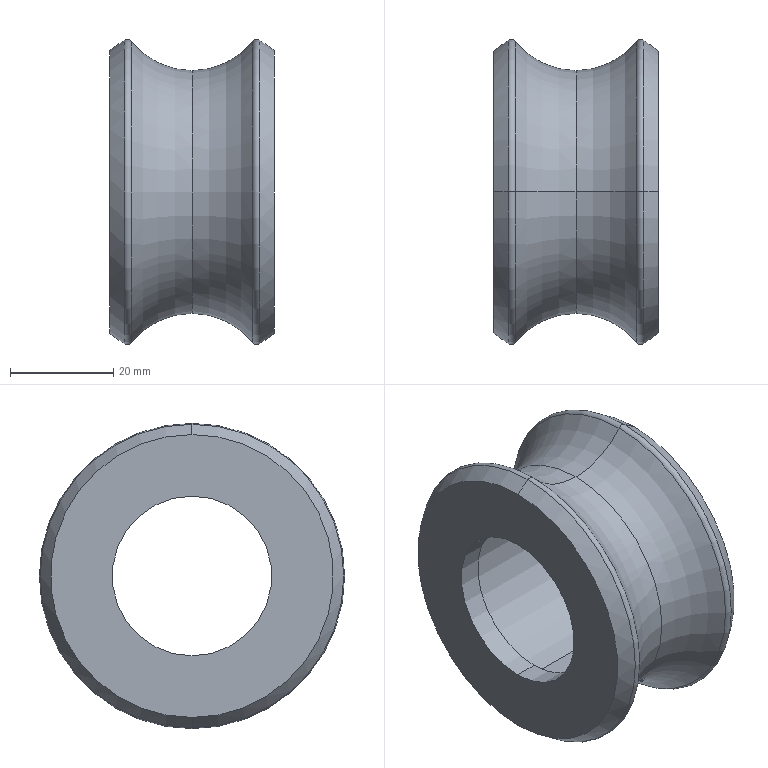Part | STEP file | RODAJA D29 | 1 solid | 29 faces | box 32 x 59.25 x 59.25 mm | volume 39424 mm3 | torus 10 | cylinder 8 | cone 6 | plane 5 | commonest cylinder face diameters 35 x4 31 x2 37.2 x2
STEP:
#1=CARTESIAN_POINT('',(-11.807,0.,-26.413));
#2=VERTEX_POINT('',#1);
#3=CARTESIAN_POINT('',(0.,0.,-32.1));
#4=VERTEX_POINT('',#3);
#5=CARTESIAN_POINT('',(0.,0.,-17.));
#6=DIRECTION('',(0.,-1.,0.));
#7=DIRECTION('',(0.,0.,-1.));
#8=AXIS2_PLACEMENT_3D('',#5,#6,#7);
#9=CIRCLE('',#8,15.1);
#10=EDGE_CURVE('',#2,#4,#9,.T.);
#11=ORIENTED_EDGE('',*,*,#10,.T.);
#12=CARTESIAN_POINT('',(0.,0.,-79.222));
#13=VERTEX_POINT('',#12);
#14=CARTESIAN_POINT('',(0.,0.,-55.661));
#15=DIRECTION('',(-1.,0.,0.));
#16=DIRECTION('',(0.,0.,1.));
#17=AXIS2_PLACEMENT_3D('',#14,#15,#16);
#18=CIRCLE('',#17,23.561);
#19=EDGE_CURVE('',#4,#13,#18,.T.);
#20=ORIENTED_EDGE('',*,*,#19,.T.);
#21=CARTESIAN_POINT('',(-11.807,0.,-84.909));
#22=VERTEX_POINT('',#21);
#23=CARTESIAN_POINT('',(0.,0.,-94.322));
#24=DIRECTION('',(0.,1.,0.));
#25=DIRECTION('',(0.,0.,1.));
#26=AXIS2_PLACEMENT_3D('',#23,#24,#25);
#27=CIRCLE('',#26,15.1);
#28=EDGE_CURVE('',#22,#13,#27,.T.);
#29=ORIENTED_EDGE('',*,*,#28,.F.);
#30=CARTESIAN_POINT('',(-11.807,0.,-55.661));
#31=DIRECTION('',(1.,0.,0.));
#32=DIRECTION('',(0.,0.,-1.));
#33=AXIS2_PLACEMENT_3D('',#30,#31,#32);
#34=CIRCLE('',#33,29.248);
#35=EDGE_CURVE('',#22,#2,#34,.T.);
#36=ORIENTED_EDGE('',*,*,#35,.T.);
#37=EDGE_LOOP('',(#11,#20,#29,#36));
#38=FACE_OUTER_BOUND('',#37,.T.);
#39=CARTESIAN_POINT('',(0.,0.,-55.661));
#40=DIRECTION('',(-1.,0.,0.));
#41=DIRECTION('',(0.,0.,1.));
#42=AXIS2_PLACEMENT_3D('',#39,#40,#41);
#43=TOROIDAL_SURFACE('',#42,38.661,15.1);
#44=ADVANCED_FACE('',(#38),#43,.F.);
#45=ORIENTED_EDGE('',*,*,#28,.T.);
#46=CARTESIAN_POINT('',(0.,0.,-55.661));
#47=DIRECTION('',(-1.,0.,0.));
#48=DIRECTION('',(0.,0.,1.));
#49=AXIS2_PLACEMENT_3D('',#46,#47,#48);
#50=CIRCLE('',#49,23.561);
#51=EDGE_CURVE('',#13,#4,#50,.T.);
#52=ORIENTED_EDGE('',*,*,#51,.T.);
#53=ORIENTED_EDGE('',*,*,#10,.F.);
#54=CARTESIAN_POINT('',(-11.807,0.,-55.661));
#55=DIRECTION('',(1.,0.,0.));
#56=DIRECTION('',(0.,0.,-1.));
#57=AXIS2_PLACEMENT_3D('',#54,#55,#56);
#58=CIRCLE('',#57,29.248);
#59=EDGE_CURVE('',#2,#22,#58,.T.);
#60=ORIENTED_EDGE('',*,*,#59,.T.);
#61=EDGE_LOOP('',(#45,#52,#53,#60));
#62=FACE_OUTER_BOUND('',#61,.T.);
#63=CARTESIAN_POINT('',(0.,0.,-55.661));
#64=DIRECTION('',(-1.,0.,0.));
#65=DIRECTION('',(0.,0.,1.));
#66=AXIS2_PLACEMENT_3D('',#63,#64,#65);
#67=TOROIDAL_SURFACE('',#66,38.661,15.1);
#68=ADVANCED_FACE('',(#62),#67,.F.);
#69=CARTESIAN_POINT('',(11.8,0.,-37.061));
#70=VERTEX_POINT('',#69);
#71=CARTESIAN_POINT('',(11.8,0.,-74.261));
#72=VERTEX_POINT('',#71);
#73=CARTESIAN_POINT('',(11.8,0.,-55.661));
#74=DIRECTION('',(1.,0.,0.));
#75=DIRECTION('',(0.,0.,-1.));
#76=AXIS2_PLACEMENT_3D('',#73,#74,#75);
#77=CIRCLE('',#76,18.6);
#78=EDGE_CURVE('',#70,#72,#77,.T.);
#79=ORIENTED_EDGE('',*,*,#78,.F.);
#80=CARTESIAN_POINT('',(13.3,0.,-37.061));
#81=VERTEX_POINT('',#80);
#82=CARTESIAN_POINT('',(16.,0.,-37.061));
#83=DIRECTION('',(1.,0.,0.));
#84=VECTOR('',#83,1000.);
#85=LINE('',#82,#84);
#86=EDGE_CURVE('',#70,#81,#85,.T.);
#87=ORIENTED_EDGE('',*,*,#86,.T.);
#88=CARTESIAN_POINT('',(13.3,0.,-74.261));
#89=VERTEX_POINT('',#88);
#90=CARTESIAN_POINT('',(13.3,0.,-55.661));
#91=DIRECTION('',(1.,0.,0.));
#92=DIRECTION('',(0.,0.,-1.));
#93=AXIS2_PLACEMENT_3D('',#90,#91,#92);
#94=CIRCLE('',#93,18.6);
#95=EDGE_CURVE('',#81,#89,#94,.T.);
#96=ORIENTED_EDGE('',*,*,#95,.T.);
#97=CARTESIAN_POINT('',(16.,0.,-74.261));
#98=DIRECTION('',(1.,0.,0.));
#99=VECTOR('',#98,1000.);
#100=LINE('',#97,#99);
#101=EDGE_CURVE('',#72,#89,#100,.T.);
#102=ORIENTED_EDGE('',*,*,#101,.F.);
#103=EDGE_LOOP('',(#79,#87,#96,#102));
#104=FACE_OUTER_BOUND('',#103,.T.);
#105=CARTESIAN_POINT('',(16.,0.,-55.661));
#106=DIRECTION('',(1.,0.,0.));
#107=DIRECTION('',(0.,0.,-1.));
#108=AXIS2_PLACEMENT_3D('',#105,#106,#107);
#109=CYLINDRICAL_SURFACE('',#108,18.6);
#110=ADVANCED_FACE('',(#104),#109,.F.);
#111=CARTESIAN_POINT('',(15.,0.,-38.161));
#112=VERTEX_POINT('',#111);
#113=CARTESIAN_POINT('',(15.,0.,-73.161));
#114=VERTEX_POINT('',#113);
#115=CARTESIAN_POINT('',(15.,0.,-55.661));
#116=DIRECTION('',(1.,0.,0.));
#117=DIRECTION('',(0.,0.,-1.));
#118=AXIS2_PLACEMENT_3D('',#115,#116,#117);
#119=CIRCLE('',#118,17.5);
#120=EDGE_CURVE('',#112,#114,#119,.T.);
#121=ORIENTED_EDGE('',*,*,#120,.F.);
#122=CARTESIAN_POINT('',(16.,0.,-37.584));
#123=VERTEX_POINT('',#122);
#124=CARTESIAN_POINT('',(15.,0.,-38.161));
#125=DIRECTION('',(0.866,0.,0.5));
#126=VECTOR('',#125,1000.);
#127=LINE('',#124,#126);
#128=EDGE_CURVE('',#112,#123,#127,.T.);
#129=ORIENTED_EDGE('',*,*,#128,.T.);
#130=CARTESIAN_POINT('',(16.,0.,-73.738));
#131=VERTEX_POINT('',#130);
#132=CARTESIAN_POINT('',(16.,0.,-55.661));
#133=DIRECTION('',(-1.,0.,0.));
#134=DIRECTION('',(0.,0.,-1.));
#135=AXIS2_PLACEMENT_3D('',#132,#133,#134);
#136=CIRCLE('',#135,18.077);
#137=EDGE_CURVE('',#131,#123,#136,.T.);
#138=ORIENTED_EDGE('',*,*,#137,.F.);
#139=CARTESIAN_POINT('',(15.,0.,-73.161));
#140=DIRECTION('',(0.866,0.,-0.5));
#141=VECTOR('',#140,1000.);
#142=LINE('',#139,#141);
#143=EDGE_CURVE('',#114,#131,#142,.T.);
#144=ORIENTED_EDGE('',*,*,#143,.F.);
#145=EDGE_LOOP('',(#121,#129,#138,#144));
#146=FACE_OUTER_BOUND('',#145,.T.);
#147=CARTESIAN_POINT('',(15.,0.,-55.661));
#148=DIRECTION('',(1.,0.,0.));
#149=DIRECTION('',(0.,0.,-1.));
#150=AXIS2_PLACEMENT_3D('',#147,#148,#149);
#151=CONICAL_SURFACE('',#150,17.5,0.5236);
#152=ADVANCED_FACE('',(#146),#151,.F.);
#153=CARTESIAN_POINT('',(-16.,0.,-71.161));
#154=VERTEX_POINT('',#153);
#155=CARTESIAN_POINT('',(-16.,0.,-40.161));
#156=VERTEX_POINT('',#155);
#157=CARTESIAN_POINT('',(-16.,0.,-55.661));
#158=DIRECTION('',(-1.,0.,0.));
#159=DIRECTION('',(0.,0.,1.));
#160=AXIS2_PLACEMENT_3D('',#157,#158,#159);
#161=CIRCLE('',#160,15.5);
#162=EDGE_CURVE('',#154,#156,#161,.T.);
#163=ORIENTED_EDGE('',*,*,#162,.T.);
#164=CARTESIAN_POINT('',(-11.5,0.,-40.161));
#165=VERTEX_POINT('',#164);
#166=CARTESIAN_POINT('',(-39.,0.,-40.161));
#167=DIRECTION('',(1.,0.,0.));
#168=VECTOR('',#167,1000.);
#169=LINE('',#166,#168);
#170=EDGE_CURVE('',#156,#165,#169,.T.);
#171=ORIENTED_EDGE('',*,*,#170,.T.);
#172=CARTESIAN_POINT('',(-11.5,0.,-71.161));
#173=VERTEX_POINT('',#172);
#174=CARTESIAN_POINT('',(-11.5,0.,-55.661));
#175=DIRECTION('',(1.,0.,0.));
#176=DIRECTION('',(0.,0.,-1.));
#177=AXIS2_PLACEMENT_3D('',#174,#175,#176);
#178=CIRCLE('',#177,15.5);
#179=EDGE_CURVE('',#165,#173,#178,.T.);
#180=ORIENTED_EDGE('',*,*,#179,.T.);
#181=CARTESIAN_POINT('',(-39.,0.,-71.161));
#182=DIRECTION('',(1.,0.,0.));
#183=VECTOR('',#182,1000.);
#184=LINE('',#181,#183);
#185=EDGE_CURVE('',#154,#173,#184,.T.);
#186=ORIENTED_EDGE('',*,*,#185,.F.);
#187=EDGE_LOOP('',(#163,#171,#180,#186));
#188=FACE_OUTER_BOUND('',#187,.T.);
#189=CARTESIAN_POINT('',(-39.,0.,-55.661));
#190=DIRECTION('',(1.,0.,0.));
#191=DIRECTION('',(0.,0.,-1.));
#192=AXIS2_PLACEMENT_3D('',#189,#190,#191);
#193=CYLINDRICAL_SURFACE('',#192,15.5);
#194=ADVANCED_FACE('',(#188),#193,.F.);
#195=CARTESIAN_POINT('',(-11.5,0.,-38.361));
#196=VERTEX_POINT('',#195);
#197=CARTESIAN_POINT('',(-11.5,0.,-72.961));
#198=VERTEX_POINT('',#197);
#199=CARTESIAN_POINT('',(-11.5,0.,-55.661));
#200=DIRECTION('',(1.,0.,0.));
#201=DIRECTION('',(0.,0.,-1.));
#202=AXIS2_PLACEMENT_3D('',#199,#200,#201);
#203=CIRCLE('',#202,17.3);
#204=EDGE_CURVE('',#196,#198,#203,.T.);
#205=ORIENTED_EDGE('',*,*,#204,.F.);
#206=CARTESIAN_POINT('',(-11.3,0.,-38.161));
#207=VERTEX_POINT('',#206);
#208=CARTESIAN_POINT('',(-11.3,0.,-38.361));
#209=DIRECTION('',(0.,1.,0.));
#210=DIRECTION('',(0.,0.,1.));
#211=AXIS2_PLACEMENT_3D('',#208,#209,#210);
#212=CIRCLE('',#211,0.2);
#213=EDGE_CURVE('',#196,#207,#212,.T.);
#214=ORIENTED_EDGE('',*,*,#213,.T.);
#215=CARTESIAN_POINT('',(-11.3,0.,-73.161));
#216=VERTEX_POINT('',#215);
#217=CARTESIAN_POINT('',(-11.3,0.,-55.661));
#218=DIRECTION('',(-1.,0.,0.));
#219=DIRECTION('',(0.,0.,-1.));
#220=AXIS2_PLACEMENT_3D('',#217,#218,#219);
#221=CIRCLE('',#220,17.5);
#222=EDGE_CURVE('',#216,#207,#221,.T.);
#223=ORIENTED_EDGE('',*,*,#222,.F.);
#224=CARTESIAN_POINT('',(-11.3,0.,-72.961));
#225=DIRECTION('',(0.,-1.,0.));
#226=DIRECTION('',(0.,0.,-1.));
#227=AXIS2_PLACEMENT_3D('',#224,#225,#226);
#228=CIRCLE('',#227,0.2);
#229=EDGE_CURVE('',#198,#216,#228,.T.);
#230=ORIENTED_EDGE('',*,*,#229,.F.);
#231=EDGE_LOOP('',(#205,#214,#223,#230));
#232=FACE_OUTER_BOUND('',#231,.T.);
#233=CARTESIAN_POINT('',(-11.3,0.,-55.661));
#234=DIRECTION('',(1.,0.,0.));
#235=DIRECTION('',(0.,0.,-1.));
#236=AXIS2_PLACEMENT_3D('',#233,#234,#235);
#237=TOROIDAL_SURFACE('',#236,17.3,0.2);
#238=ADVANCED_FACE('',(#232),#237,.F.);
#239=CARTESIAN_POINT('',(13.3,0.,-73.161));
#240=VERTEX_POINT('',#239);
#241=CARTESIAN_POINT('',(13.3,0.,-38.161));
#242=VERTEX_POINT('',#241);
#243=CARTESIAN_POINT('',(13.3,0.,-55.661));
#244=DIRECTION('',(-1.,0.,0.));
#245=DIRECTION('',(0.,0.,-1.));
#246=AXIS2_PLACEMENT_3D('',#243,#244,#245);
#247=CIRCLE('',#246,17.5);
#248=EDGE_CURVE('',#240,#242,#247,.T.);
#249=ORIENTED_EDGE('',*,*,#248,.T.);
#250=CARTESIAN_POINT('',(-11.5,0.,-38.161));
#251=DIRECTION('',(1.,0.,0.));
#252=VECTOR('',#251,1000.);
#253=LINE('',#250,#252);
#254=EDGE_CURVE('',#242,#112,#253,.T.);
#255=ORIENTED_EDGE('',*,*,#254,.T.);
#256=ORIENTED_EDGE('',*,*,#120,.T.);
#257=CARTESIAN_POINT('',(-11.5,0.,-73.161));
#258=DIRECTION('',(1.,0.,0.));
#259=VECTOR('',#258,1000.);
#260=LINE('',#257,#259);
#261=EDGE_CURVE('',#240,#114,#260,.T.);
#262=ORIENTED_EDGE('',*,*,#261,.F.);
#263=EDGE_LOOP('',(#249,#255,#256,#262));
#264=FACE_OUTER_BOUND('',#263,.T.);
#265=CARTESIAN_POINT('',(-11.5,0.,-55.661));
#266=DIRECTION('',(1.,0.,0.));
#267=DIRECTION('',(0.,0.,-1.));
#268=AXIS2_PLACEMENT_3D('',#265,#266,#267);
#269=CYLINDRICAL_SURFACE('',#268,17.5);
#270=ADVANCED_FACE('',(#264),#269,.F.);
#271=CARTESIAN_POINT('',(-13.163,0.,-26.217));
#272=VERTEX_POINT('',#271);
#273=CARTESIAN_POINT('',(-13.163,0.,-85.105));
#274=VERTEX_POINT('',#273);
#275=CARTESIAN_POINT('',(-13.163,0.,-55.661));
#276=DIRECTION('',(-1.,0.,0.));
#277=DIRECTION('',(0.,0.,1.));
#278=AXIS2_PLACEMENT_3D('',#275,#276,#277);
#279=CIRCLE('',#278,29.444);
#280=EDGE_CURVE('',#272,#274,#279,.T.);
#281=ORIENTED_EDGE('',*,*,#280,.F.);
#282=CARTESIAN_POINT('',(-12.589,0.,-27.036));
#283=DIRECTION('',(0.,1.,0.));
#284=DIRECTION('',(0.,0.,1.));
#285=AXIS2_PLACEMENT_3D('',#282,#283,#284);
#286=CIRCLE('',#285,1.);
#287=EDGE_CURVE('',#272,#2,#286,.T.);
#288=ORIENTED_EDGE('',*,*,#287,.T.);
#289=ORIENTED_EDGE('',*,*,#35,.F.);
#290=CARTESIAN_POINT('',(-12.589,0.,-84.286));
#291=DIRECTION('',(0.,-1.,0.));
#292=DIRECTION('',(0.,0.,-1.));
#293=AXIS2_PLACEMENT_3D('',#290,#291,#292);
#294=CIRCLE('',#293,1.);
#295=EDGE_CURVE('',#274,#22,#294,.T.);
#296=ORIENTED_EDGE('',*,*,#295,.F.);
#297=EDGE_LOOP('',(#281,#288,#289,#296));
#298=FACE_OUTER_BOUND('',#297,.T.);
#299=CARTESIAN_POINT('',(-12.589,0.,-55.661));
#300=DIRECTION('',(1.,0.,0.));
#301=DIRECTION('',(0.,0.,-1.));
#302=AXIS2_PLACEMENT_3D('',#299,#300,#301);
#303=TOROIDAL_SURFACE('',#302,28.625,1.);
#304=ADVANCED_FACE('',(#298),#303,.T.);
#305=CARTESIAN_POINT('',(11.807,0.,-26.413));
#306=VERTEX_POINT('',#305);
#307=CARTESIAN_POINT('',(11.807,0.,-84.909));
#308=VERTEX_POINT('',#307);
#309=CARTESIAN_POINT('',(11.807,0.,-55.661));
#310=DIRECTION('',(-1.,0.,0.));
#311=DIRECTION('',(0.,0.,1.));
#312=AXIS2_PLACEMENT_3D('',#309,#310,#311);
#313=CIRCLE('',#312,29.248);
#314=EDGE_CURVE('',#306,#308,#313,.T.);
#315=ORIENTED_EDGE('',*,*,#314,.F.);
#316=CARTESIAN_POINT('',(13.163,0.,-26.217));
#317=VERTEX_POINT('',#316);
#318=CARTESIAN_POINT('',(12.589,0.,-27.036));
#319=DIRECTION('',(0.,1.,0.));
#320=DIRECTION('',(0.,0.,1.));
#321=AXIS2_PLACEMENT_3D('',#318,#319,#320);
#322=CIRCLE('',#321,1.);
#323=EDGE_CURVE('',#306,#317,#322,.T.);
#324=ORIENTED_EDGE('',*,*,#323,.T.);
#325=CARTESIAN_POINT('',(13.163,0.,-85.105));
#326=VERTEX_POINT('',#325);
#327=CARTESIAN_POINT('',(13.163,0.,-55.661));
#328=DIRECTION('',(1.,0.,0.));
#329=DIRECTION('',(0.,0.,-1.));
#330=AXIS2_PLACEMENT_3D('',#327,#328,#329);
#331=CIRCLE('',#330,29.444);
#332=EDGE_CURVE('',#326,#317,#331,.T.);
#333=ORIENTED_EDGE('',*,*,#332,.F.);
#334=CARTESIAN_POINT('',(12.589,0.,-84.286));
#335=DIRECTION('',(0.,-1.,0.));
#336=DIRECTION('',(0.,0.,-1.));
#337=AXIS2_PLACEMENT_3D('',#334,#335,#336);
#338=CIRCLE('',#337,1.);
#339=EDGE_CURVE('',#308,#326,#338,.T.);
#340=ORIENTED_EDGE('',*,*,#339,.F.);
#341=EDGE_LOOP('',(#315,#324,#333,#340));
#342=FACE_OUTER_BOUND('',#341,.T.);
#343=CARTESIAN_POINT('',(12.589,0.,-55.661));
#344=DIRECTION('',(1.,0.,0.));
#345=DIRECTION('',(0.,0.,-1.));
#346=AXIS2_PLACEMENT_3D('',#343,#344,#345);
#347=TOROIDAL_SURFACE('',#346,28.625,1.);
#348=ADVANCED_FACE('',(#342),#347,.T.);
#349=CARTESIAN_POINT('',(16.,0.,-28.203));
#350=VERTEX_POINT('',#349);
#351=CARTESIAN_POINT('',(16.,0.,-83.119));
#352=VERTEX_POINT('',#351);
#353=CARTESIAN_POINT('',(16.,0.,-55.661));
#354=DIRECTION('',(-1.,0.,0.));
#355=DIRECTION('',(0.,0.,1.));
#356=AXIS2_PLACEMENT_3D('',#353,#354,#355);
#357=CIRCLE('',#356,27.458);
#358=EDGE_CURVE('',#350,#352,#357,.T.);
#359=ORIENTED_EDGE('',*,*,#358,.T.);
#360=CARTESIAN_POINT('',(12.369,0.,-85.661));
#361=DIRECTION('',(-0.8192,0.,-0.5736));
#362=VECTOR('',#361,1000.);
#363=LINE('',#360,#362);
#364=EDGE_CURVE('',#352,#326,#363,.T.);
#365=ORIENTED_EDGE('',*,*,#364,.T.);
#366=ORIENTED_EDGE('',*,*,#332,.T.);
#367=CARTESIAN_POINT('',(12.369,0.,-25.661));
#368=DIRECTION('',(-0.8192,0.,0.5736));
#369=VECTOR('',#368,1000.);
#370=LINE('',#367,#369);
#371=EDGE_CURVE('',#350,#317,#370,.T.);
#372=ORIENTED_EDGE('',*,*,#371,.F.);
#373=EDGE_LOOP('',(#359,#365,#366,#372));
#374=FACE_OUTER_BOUND('',#373,.T.);
#375=CARTESIAN_POINT('',(12.369,0.,-55.661));
#376=DIRECTION('',(-1.,0.,0.));
#377=DIRECTION('',(0.,0.,1.));
#378=AXIS2_PLACEMENT_3D('',#375,#376,#377);
#379=CONICAL_SURFACE('',#378,30.,0.6109);
#380=ADVANCED_FACE('',(#374),#379,.T.);
#381=CARTESIAN_POINT('',(-16.,0.,-28.203));
#382=VERTEX_POINT('',#381);
#383=CARTESIAN_POINT('',(-16.,0.,-83.119));
#384=VERTEX_POINT('',#383);
#385=CARTESIAN_POINT('',(-16.,0.,-55.661));
#386=DIRECTION('',(-1.,0.,0.));
#387=DIRECTION('',(0.,0.,1.));
#388=AXIS2_PLACEMENT_3D('',#385,#386,#387);
#389=CIRCLE('',#388,27.458);
#390=EDGE_CURVE('',#382,#384,#389,.T.);
#391=ORIENTED_EDGE('',*,*,#390,.F.);
#392=CARTESIAN_POINT('',(-16.,0.,-28.203));
#393=DIRECTION('',(0.8192,0.,0.5736));
#394=VECTOR('',#393,1000.);
#395=LINE('',#392,#394);
#396=EDGE_CURVE('',#382,#272,#395,.T.);
#397=ORIENTED_EDGE('',*,*,#396,.T.);
#398=ORIENTED_EDGE('',*,*,#280,.T.);
#399=CARTESIAN_POINT('',(-16.,0.,-83.119));
#400=DIRECTION('',(0.8192,0.,-0.5736));
#401=VECTOR('',#400,1000.);
#402=LINE('',#399,#401);
#403=EDGE_CURVE('',#384,#274,#402,.T.);
#404=ORIENTED_EDGE('',*,*,#403,.F.);
#405=EDGE_LOOP('',(#391,#397,#398,#404));
#406=FACE_OUTER_BOUND('',#405,.T.);
#407=CARTESIAN_POINT('',(-16.,0.,-55.661));
#408=DIRECTION('',(1.,0.,0.));
#409=DIRECTION('',(0.,0.,-1.));
#410=AXIS2_PLACEMENT_3D('',#407,#408,#409);
#411=CONICAL_SURFACE('',#410,27.458,0.6109);
#412=ADVANCED_FACE('',(#406),#411,.T.);
#413=ORIENTED_EDGE('',*,*,#51,.F.);
#414=CARTESIAN_POINT('',(0.,0.,-94.322));
#415=DIRECTION('',(0.,1.,0.));
#416=DIRECTION('',(0.,0.,1.));
#417=AXIS2_PLACEMENT_3D('',#414,#415,#416);
#418=CIRCLE('',#417,15.1);
#419=EDGE_CURVE('',#13,#308,#418,.T.);
#420=ORIENTED_EDGE('',*,*,#419,.T.);
#421=CARTESIAN_POINT('',(11.807,0.,-55.661));
#422=DIRECTION('',(-1.,0.,0.));
#423=DIRECTION('',(0.,0.,1.));
#424=AXIS2_PLACEMENT_3D('',#421,#422,#423);
#425=CIRCLE('',#424,29.248);
#426=EDGE_CURVE('',#308,#306,#425,.T.);
#427=ORIENTED_EDGE('',*,*,#426,.T.);
#428=CARTESIAN_POINT('',(0.,0.,-17.));
#429=DIRECTION('',(0.,-1.,0.));
#430=DIRECTION('',(0.,0.,-1.));
#431=AXIS2_PLACEMENT_3D('',#428,#429,#430);
#432=CIRCLE('',#431,15.1);
#433=EDGE_CURVE('',#4,#306,#432,.T.);
#434=ORIENTED_EDGE('',*,*,#433,.F.);
#435=EDGE_LOOP('',(#413,#420,#427,#434));
#436=FACE_OUTER_BOUND('',#435,.T.);
#437=CARTESIAN_POINT('',(0.,0.,-55.661));
#438=DIRECTION('',(-1.,0.,0.));
#439=DIRECTION('',(0.,0.,1.));
#440=AXIS2_PLACEMENT_3D('',#437,#438,#439);
#441=TOROIDAL_SURFACE('',#440,38.661,15.1);
#442=ADVANCED_FACE('',(#436),#441,.F.);
#443=ORIENTED_EDGE('',*,*,#222,.T.);
#444=CARTESIAN_POINT('',(11.8,0.,-38.161));
#445=VERTEX_POINT('',#444);
#446=CARTESIAN_POINT('',(-11.5,0.,-38.161));
#447=DIRECTION('',(1.,0.,0.));
#448=VECTOR('',#447,1000.);
#449=LINE('',#446,#448);
#450=EDGE_CURVE('',#207,#445,#449,.T.);
#451=ORIENTED_EDGE('',*,*,#450,.T.);
#452=CARTESIAN_POINT('',(11.8,0.,-73.161));
#453=VERTEX_POINT('',#452);
#454=CARTESIAN_POINT('',(11.8,0.,-55.661));
#455=DIRECTION('',(1.,0.,0.));
#456=DIRECTION('',(0.,0.,1.));
#457=AXIS2_PLACEMENT_3D('',#454,#455,#456);
#458=CIRCLE('',#457,17.5);
#459=EDGE_CURVE('',#445,#453,#458,.T.);
#460=ORIENTED_EDGE('',*,*,#459,.T.);
#461=CARTESIAN_POINT('',(-11.5,0.,-73.161));
#462=DIRECTION('',(1.,0.,0.));
#463=VECTOR('',#462,1000.);
#464=LINE('',#461,#463);
#465=EDGE_CURVE('',#216,#453,#464,.T.);
#466=ORIENTED_EDGE('',*,*,#465,.F.);
#467=EDGE_LOOP('',(#443,#451,#460,#466));
#468=FACE_OUTER_BOUND('',#467,.T.);
#469=CARTESIAN_POINT('',(-11.5,0.,-55.661));
#470=DIRECTION('',(1.,0.,0.));
#471=DIRECTION('',(0.,0.,-1.));
#472=AXIS2_PLACEMENT_3D('',#469,#470,#471);
#473=CYLINDRICAL_SURFACE('',#472,17.5);
#474=ADVANCED_FACE('',(#468),#473,.F.);
#475=ORIENTED_EDGE('',*,*,#450,.F.);
#476=CARTESIAN_POINT('',(-11.3,0.,-55.661));
#477=DIRECTION('',(-1.,0.,0.));
#478=DIRECTION('',(0.,0.,-1.));
#479=AXIS2_PLACEMENT_3D('',#476,#477,#478);
#480=CIRCLE('',#479,17.5);
#481=EDGE_CURVE('',#207,#216,#480,.T.);
#482=ORIENTED_EDGE('',*,*,#481,.T.);
#483=ORIENTED_EDGE('',*,*,#465,.T.);
#484=CARTESIAN_POINT('',(11.8,0.,-55.661));
#485=DIRECTION('',(1.,0.,0.));
#486=DIRECTION('',(0.,0.,1.));
#487=AXIS2_PLACEMENT_3D('',#484,#485,#486);
#488=CIRCLE('',#487,17.5);
#489=EDGE_CURVE('',#453,#445,#488,.T.);
#490=ORIENTED_EDGE('',*,*,#489,.T.);
#491=EDGE_LOOP('',(#475,#482,#483,#490));
#492=FACE_OUTER_BOUND('',#491,.T.);
#493=CARTESIAN_POINT('',(-11.5,0.,-55.661));
#494=DIRECTION('',(1.,0.,0.));
#495=DIRECTION('',(0.,0.,-1.));
#496=AXIS2_PLACEMENT_3D('',#493,#494,#495);
#497=CYLINDRICAL_SURFACE('',#496,17.5);
#498=ADVANCED_FACE('',(#492),#497,.F.);
#499=ORIENTED_EDGE('',*,*,#19,.F.);
#500=ORIENTED_EDGE('',*,*,#433,.T.);
#501=ORIENTED_EDGE('',*,*,#314,.T.);
#502=ORIENTED_EDGE('',*,*,#419,.F.);
#503=EDGE_LOOP('',(#499,#500,#501,#502));
#504=FACE_OUTER_BOUND('',#503,.T.);
#505=CARTESIAN_POINT('',(0.,0.,-55.661));
#506=DIRECTION('',(-1.,0.,0.));
#507=DIRECTION('',(0.,0.,1.));
#508=AXIS2_PLACEMENT_3D('',#505,#506,#507);
#509=TOROIDAL_SURFACE('',#508,38.661,15.1);
#510=ADVANCED_FACE('',(#504),#509,.F.);
#511=ORIENTED_EDGE('',*,*,#396,.F.);
#512=CARTESIAN_POINT('',(-16.,0.,-55.661));
#513=DIRECTION('',(-1.,0.,0.));
#514=DIRECTION('',(0.,0.,1.));
#515=AXIS2_PLACEMENT_3D('',#512,#513,#514);
#516=CIRCLE('',#515,27.458);
#517=EDGE_CURVE('',#384,#382,#516,.T.);
#518=ORIENTED_EDGE('',*,*,#517,.F.);
#519=ORIENTED_EDGE('',*,*,#403,.T.);
#520=CARTESIAN_POINT('',(-13.163,0.,-55.661));
#521=DIRECTION('',(-1.,0.,0.));
#522=DIRECTION('',(0.,0.,1.));
#523=AXIS2_PLACEMENT_3D('',#520,#521,#522);
#524=CIRCLE('',#523,29.444);
#525=EDGE_CURVE('',#274,#272,#524,.T.);
#526=ORIENTED_EDGE('',*,*,#525,.T.);
#527=EDGE_LOOP('',(#511,#518,#519,#526));
#528=FACE_OUTER_BOUND('',#527,.T.);
#529=CARTESIAN_POINT('',(-16.,0.,-55.661));
#530=DIRECTION('',(1.,0.,0.));
#531=DIRECTION('',(0.,0.,-1.));
#532=AXIS2_PLACEMENT_3D('',#529,#530,#531);
#533=CONICAL_SURFACE('',#532,27.458,0.6109);
#534=ADVANCED_FACE('',(#528),#533,.T.);
#535=ORIENTED_EDGE('',*,*,#162,.F.);
#536=CARTESIAN_POINT('',(-16.,0.,-55.661));
#537=DIRECTION('',(-1.,0.,0.));
#538=DIRECTION('',(0.,0.,1.));
#539=AXIS2_PLACEMENT_3D('',#536,#537,#538);
#540=CIRCLE('',#539,15.5);
#541=EDGE_CURVE('',#156,#154,#540,.T.);
#542=ORIENTED_EDGE('',*,*,#541,.F.);
#543=EDGE_LOOP('',(#535,#542));
#544=FACE_BOUND('',#543,.T.);
#545=ORIENTED_EDGE('',*,*,#517,.T.);
#546=ORIENTED_EDGE('',*,*,#390,.T.);
#547=EDGE_LOOP('',(#545,#546));
#548=FACE_OUTER_BOUND('',#547,.T.);
#549=CARTESIAN_POINT('',(-16.,0.,-28.203));
#550=DIRECTION('',(-1.,0.,0.));
#551=DIRECTION('',(0.,0.,1.));
#552=AXIS2_PLACEMENT_3D('',#549,#550,#551);
#553=PLANE('',#552);
#554=ADVANCED_FACE('',(#544,#548),#553,.T.);
#555=ORIENTED_EDGE('',*,*,#137,.T.);
#556=CARTESIAN_POINT('',(16.,0.,-55.661));
#557=DIRECTION('',(-1.,0.,0.));
#558=DIRECTION('',(0.,0.,-1.));
#559=AXIS2_PLACEMENT_3D('',#556,#557,#558);
#560=CIRCLE('',#559,18.077);
#561=EDGE_CURVE('',#123,#131,#560,.T.);
#562=ORIENTED_EDGE('',*,*,#561,.T.);
#563=EDGE_LOOP('',(#555,#562));
#564=FACE_BOUND('',#563,.T.);
#565=ORIENTED_EDGE('',*,*,#358,.F.);
#566=CARTESIAN_POINT('',(16.,0.,-55.661));
#567=DIRECTION('',(-1.,0.,0.));
#568=DIRECTION('',(0.,0.,1.));
#569=AXIS2_PLACEMENT_3D('',#566,#567,#568);
#570=CIRCLE('',#569,27.458);
#571=EDGE_CURVE('',#352,#350,#570,.T.);
#572=ORIENTED_EDGE('',*,*,#571,.F.);
#573=EDGE_LOOP('',(#565,#572));
#574=FACE_OUTER_BOUND('',#573,.T.);
#575=CARTESIAN_POINT('',(16.,0.,-28.203));
#576=DIRECTION('',(1.,0.,0.));
#577=DIRECTION('',(0.,0.,-1.));
#578=AXIS2_PLACEMENT_3D('',#575,#576,#577);
#579=PLANE('',#578);
#580=ADVANCED_FACE('',(#564,#574),#579,.T.);
#581=ORIENTED_EDGE('',*,*,#364,.F.);
#582=ORIENTED_EDGE('',*,*,#571,.T.);
#583=ORIENTED_EDGE('',*,*,#371,.T.);
#584=CARTESIAN_POINT('',(13.163,0.,-55.661));
#585=DIRECTION('',(1.,0.,0.));
#586=DIRECTION('',(0.,0.,-1.));
#587=AXIS2_PLACEMENT_3D('',#584,#585,#586);
#588=CIRCLE('',#587,29.444);
#589=EDGE_CURVE('',#317,#326,#588,.T.);
#590=ORIENTED_EDGE('',*,*,#589,.T.);
#591=EDGE_LOOP('',(#581,#582,#583,#590));
#592=FACE_OUTER_BOUND('',#591,.T.);
#593=CARTESIAN_POINT('',(12.369,0.,-55.661));
#594=DIRECTION('',(-1.,0.,0.));
#595=DIRECTION('',(0.,0.,1.));
#596=AXIS2_PLACEMENT_3D('',#593,#594,#595);
#597=CONICAL_SURFACE('',#596,30.,0.6109);
#598=ADVANCED_FACE('',(#592),#597,.T.);
#599=ORIENTED_EDGE('',*,*,#323,.F.);
#600=ORIENTED_EDGE('',*,*,#426,.F.);
#601=ORIENTED_EDGE('',*,*,#339,.T.);
#602=ORIENTED_EDGE('',*,*,#589,.F.);
#603=EDGE_LOOP('',(#599,#600,#601,#602));
#604=FACE_OUTER_BOUND('',#603,.T.);
#605=CARTESIAN_POINT('',(12.589,0.,-55.661));
#606=DIRECTION('',(1.,0.,0.));
#607=DIRECTION('',(0.,0.,-1.));
#608=AXIS2_PLACEMENT_3D('',#605,#606,#607);
#609=TOROIDAL_SURFACE('',#608,28.625,1.);
#610=ADVANCED_FACE('',(#604),#609,.T.);
#611=ORIENTED_EDGE('',*,*,#287,.F.);
#612=ORIENTED_EDGE('',*,*,#525,.F.);
#613=ORIENTED_EDGE('',*,*,#295,.T.);
#614=ORIENTED_EDGE('',*,*,#59,.F.);
#615=EDGE_LOOP('',(#611,#612,#613,#614));
#616=FACE_OUTER_BOUND('',#615,.T.);
#617=CARTESIAN_POINT('',(-12.589,0.,-55.661));
#618=DIRECTION('',(1.,0.,0.));
#619=DIRECTION('',(0.,0.,-1.));
#620=AXIS2_PLACEMENT_3D('',#617,#618,#619);
#621=TOROIDAL_SURFACE('',#620,28.625,1.);
#622=ADVANCED_FACE('',(#616),#621,.T.);
#623=ORIENTED_EDGE('',*,*,#254,.F.);
#624=CARTESIAN_POINT('',(13.3,0.,-55.661));
#625=DIRECTION('',(-1.,0.,0.));
#626=DIRECTION('',(0.,0.,-1.));
#627=AXIS2_PLACEMENT_3D('',#624,#625,#626);
#628=CIRCLE('',#627,17.5);
#629=EDGE_CURVE('',#242,#240,#628,.T.);
#630=ORIENTED_EDGE('',*,*,#629,.T.);
#631=ORIENTED_EDGE('',*,*,#261,.T.);
#632=CARTESIAN_POINT('',(15.,0.,-55.661));
#633=DIRECTION('',(1.,0.,0.));
#634=DIRECTION('',(0.,0.,-1.));
#635=AXIS2_PLACEMENT_3D('',#632,#633,#634);
#636=CIRCLE('',#635,17.5);
#637=EDGE_CURVE('',#114,#112,#636,.T.);
#638=ORIENTED_EDGE('',*,*,#637,.T.);
#639=EDGE_LOOP('',(#623,#630,#631,#638));
#640=FACE_OUTER_BOUND('',#639,.T.);
#641=CARTESIAN_POINT('',(-11.5,0.,-55.661));
#642=DIRECTION('',(1.,0.,0.));
#643=DIRECTION('',(0.,0.,-1.));
#644=AXIS2_PLACEMENT_3D('',#641,#642,#643);
#645=CYLINDRICAL_SURFACE('',#644,17.5);
#646=ADVANCED_FACE('',(#640),#645,.F.);
#647=CARTESIAN_POINT('',(-11.5,0.,-55.661));
#648=DIRECTION('',(1.,0.,0.));
#649=DIRECTION('',(0.,0.,-1.));
#650=AXIS2_PLACEMENT_3D('',#647,#648,#649);
#651=CIRCLE('',#650,15.5);
#652=EDGE_CURVE('',#173,#165,#651,.T.);
#653=ORIENTED_EDGE('',*,*,#652,.F.);
#654=ORIENTED_EDGE('',*,*,#179,.F.);
#655=EDGE_LOOP('',(#653,#654));
#656=FACE_BOUND('',#655,.T.);
#657=CARTESIAN_POINT('',(-11.5,0.,-55.661));
#658=DIRECTION('',(1.,0.,0.));
#659=DIRECTION('',(0.,0.,-1.));
#660=AXIS2_PLACEMENT_3D('',#657,#658,#659);
#661=CIRCLE('',#660,17.3);
#662=EDGE_CURVE('',#198,#196,#661,.T.);
#663=ORIENTED_EDGE('',*,*,#662,.T.);
#664=ORIENTED_EDGE('',*,*,#204,.T.);
#665=EDGE_LOOP('',(#663,#664));
#666=FACE_OUTER_BOUND('',#665,.T.);
#667=CARTESIAN_POINT('',(-11.5,0.,-55.661));
#668=DIRECTION('',(1.,0.,0.));
#669=DIRECTION('',(0.,0.,-1.));
#670=AXIS2_PLACEMENT_3D('',#667,#668,#669);
#671=PLANE('',#670);
#672=ADVANCED_FACE('',(#656,#666),#671,.T.);
#673=ORIENTED_EDGE('',*,*,#213,.F.);
#674=ORIENTED_EDGE('',*,*,#662,.F.);
#675=ORIENTED_EDGE('',*,*,#229,.T.);
#676=ORIENTED_EDGE('',*,*,#481,.F.);
#677=EDGE_LOOP('',(#673,#674,#675,#676));
#678=FACE_OUTER_BOUND('',#677,.T.);
#679=CARTESIAN_POINT('',(-11.3,0.,-55.661));
#680=DIRECTION('',(1.,0.,0.));
#681=DIRECTION('',(0.,0.,-1.));
#682=AXIS2_PLACEMENT_3D('',#679,#680,#681);
#683=TOROIDAL_SURFACE('',#682,17.3,0.2);
#684=ADVANCED_FACE('',(#678),#683,.F.);
#685=ORIENTED_EDGE('',*,*,#170,.F.);
#686=ORIENTED_EDGE('',*,*,#541,.T.);
#687=ORIENTED_EDGE('',*,*,#185,.T.);
#688=ORIENTED_EDGE('',*,*,#652,.T.);
#689=EDGE_LOOP('',(#685,#686,#687,#688));
#690=FACE_OUTER_BOUND('',#689,.T.);
#691=CARTESIAN_POINT('',(-39.,0.,-55.661));
#692=DIRECTION('',(1.,0.,0.));
#693=DIRECTION('',(0.,0.,-1.));
#694=AXIS2_PLACEMENT_3D('',#691,#692,#693);
#695=CYLINDRICAL_SURFACE('',#694,15.5);
#696=ADVANCED_FACE('',(#690),#695,.F.);
#697=ORIENTED_EDGE('',*,*,#128,.F.);
#698=ORIENTED_EDGE('',*,*,#637,.F.);
#699=ORIENTED_EDGE('',*,*,#143,.T.);
#700=ORIENTED_EDGE('',*,*,#561,.F.);
#701=EDGE_LOOP('',(#697,#698,#699,#700));
#702=FACE_OUTER_BOUND('',#701,.T.);
#703=CARTESIAN_POINT('',(15.,0.,-55.661));
#704=DIRECTION('',(1.,0.,0.));
#705=DIRECTION('',(0.,0.,-1.));
#706=AXIS2_PLACEMENT_3D('',#703,#704,#705);
#707=CONICAL_SURFACE('',#706,17.5,0.5236);
#708=ADVANCED_FACE('',(#702),#707,.F.);
#709=CARTESIAN_POINT('',(11.8,0.,-55.661));
#710=DIRECTION('',(1.,0.,0.));
#711=DIRECTION('',(0.,0.,-1.));
#712=AXIS2_PLACEMENT_3D('',#709,#710,#711);
#713=CIRCLE('',#712,18.6);
#714=EDGE_CURVE('',#72,#70,#713,.T.);
#715=ORIENTED_EDGE('',*,*,#714,.T.);
#716=ORIENTED_EDGE('',*,*,#78,.T.);
#717=EDGE_LOOP('',(#715,#716));
#718=FACE_OUTER_BOUND('',#717,.T.);
#719=ORIENTED_EDGE('',*,*,#489,.F.);
#720=ORIENTED_EDGE('',*,*,#459,.F.);
#721=EDGE_LOOP('',(#719,#720));
#722=FACE_BOUND('',#721,.T.);
#723=CARTESIAN_POINT('',(11.8,0.,-69.874));
#724=DIRECTION('',(-1.,0.,0.));
#725=DIRECTION('',(0.,0.,1.));
#726=AXIS2_PLACEMENT_3D('',#723,#724,#725);
#727=PLANE('',#726);
#728=ADVANCED_FACE('',(#718,#722),#727,.F.);
#729=CARTESIAN_POINT('',(13.3,0.,-55.661));
#730=DIRECTION('',(1.,0.,0.));
#731=DIRECTION('',(0.,0.,-1.));
#732=AXIS2_PLACEMENT_3D('',#729,#730,#731);
#733=CIRCLE('',#732,18.6);
#734=EDGE_CURVE('',#89,#81,#733,.T.);
#735=ORIENTED_EDGE('',*,*,#734,.F.);
#736=ORIENTED_EDGE('',*,*,#95,.F.);
#737=EDGE_LOOP('',(#735,#736));
#738=FACE_OUTER_BOUND('',#737,.T.);
#739=ORIENTED_EDGE('',*,*,#248,.F.);
#740=ORIENTED_EDGE('',*,*,#629,.F.);
#741=EDGE_LOOP('',(#739,#740));
#742=FACE_BOUND('',#741,.T.);
#743=CARTESIAN_POINT('',(13.3,0.,-69.874));
#744=DIRECTION('',(1.,0.,0.));
#745=DIRECTION('',(0.,0.,-1.));
#746=AXIS2_PLACEMENT_3D('',#743,#744,#745);
#747=PLANE('',#746);
#748=ADVANCED_FACE('',(#738,#742),#747,.F.);
#749=ORIENTED_EDGE('',*,*,#86,.F.);
#750=ORIENTED_EDGE('',*,*,#714,.F.);
#751=ORIENTED_EDGE('',*,*,#101,.T.);
#752=ORIENTED_EDGE('',*,*,#734,.T.);
#753=EDGE_LOOP('',(#749,#750,#751,#752));
#754=FACE_OUTER_BOUND('',#753,.T.);
#755=CARTESIAN_POINT('',(16.,0.,-55.661));
#756=DIRECTION('',(1.,0.,0.));
#757=DIRECTION('',(0.,0.,-1.));
#758=AXIS2_PLACEMENT_3D('',#755,#756,#757);
#759=CYLINDRICAL_SURFACE('',#758,18.6);
#760=ADVANCED_FACE('',(#754),#759,.F.);
#761=CLOSED_SHELL('',(#44,#68,#110,#152,#194,#238,#270,#304,#348,#380,#412,#442,#474,#498,#510,#534,#554,#580,#598,#610,#622,#646,#672,#684,#696,#708,#728,#748,#760));
#762=MANIFOLD_SOLID_BREP('',#761);
#763=CARTESIAN_POINT('',(0.,0.,0.));
#764=DIRECTION('',(0.,0.,1.));
#765=DIRECTION('',(1.,0.,0.));
#766=AXIS2_PLACEMENT_3D('',#763,#764,#765);
#767=(LENGTH_UNIT()NAMED_UNIT(*)SI_UNIT(.MILLI.,.METRE.));
#768=UNCERTAINTY_MEASURE_WITH_UNIT(LENGTH_MEASURE(0.00001),#767,'','');
#769=(NAMED_UNIT(*)PLANE_ANGLE_UNIT()SI_UNIT($,.RADIAN.));
#770=(NAMED_UNIT(*)SI_UNIT($,.STERADIAN.)SOLID_ANGLE_UNIT());
#771=(GEOMETRIC_REPRESENTATION_CONTEXT(3)GLOBAL_UNCERTAINTY_ASSIGNED_CONTEXT((#768))GLOBAL_UNIT_ASSIGNED_CONTEXT((#767,#769,#770))REPRESENTATION_CONTEXT('',''));
#772=ADVANCED_BREP_SHAPE_REPRESENTATION('',(#762,#766),#771);